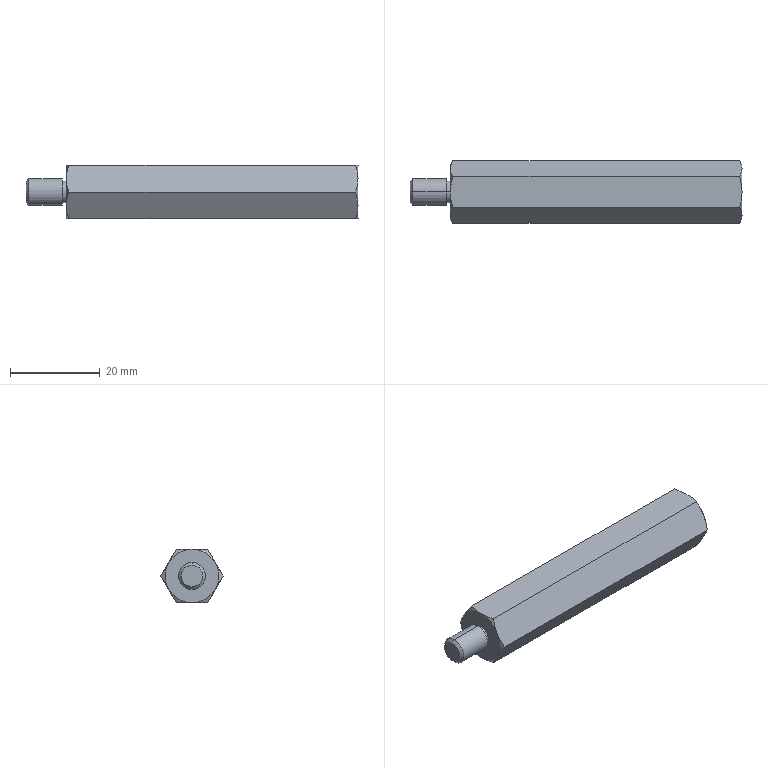Part | STEP file | 0245_024_PLSBWF12-65 | 1 solid | 34 faces | box 74 x 13.856 x 12 mm | volume 8075 mm3 | cone 18 | plane 10 | cylinder 6 | commonest cylinder face diameters 4.8 x2 4.917 x2 6 x2